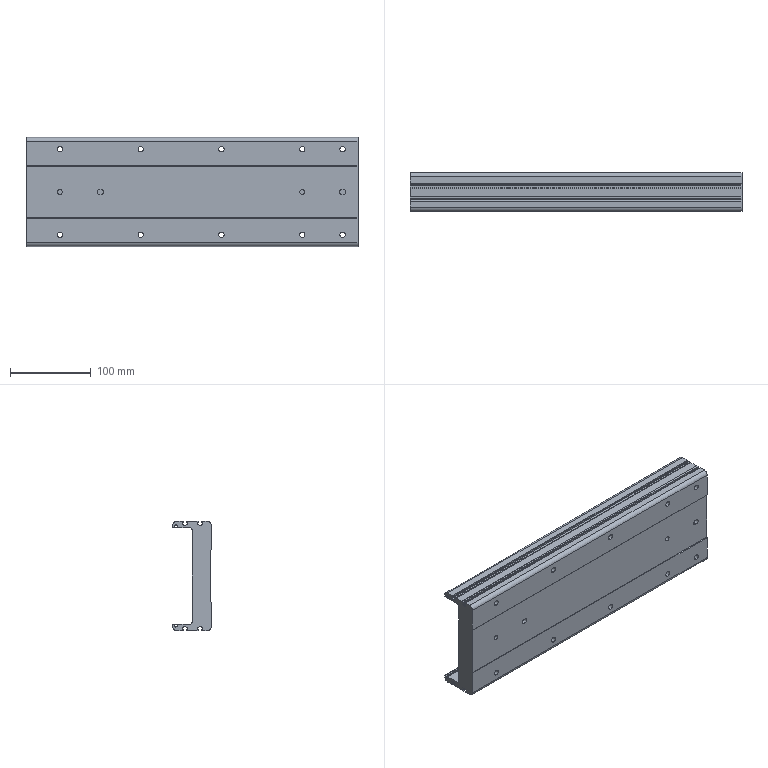Part | SolidWorks | features BaseBody 1 | 1 solid | 181 faces | box 411 x 48 x 135 mm | volume 1401649 mm3 | plane 92 | cylinder 69 | cone 20 | commonest cylinder face diameters 6.647 x20 11 x20 6 x8 4.2 x6 0.4 x4 10 x4